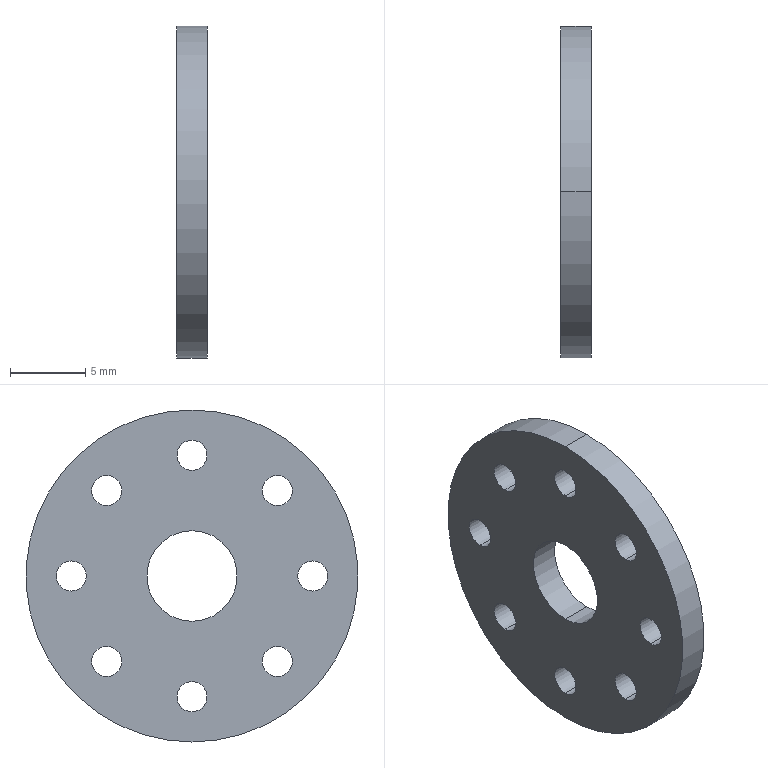Part | SolidWorks | features BaseBody 1 | 1 solid | 22 faces | box 2 x 22 x 22 mm | volume 653.451 mm3 | cylinder 20 | plane 2 | commonest cylinder face diameters 2 x16 6 x2 22 x2
STEP:
#1=CARTESIAN_POINT('',(1.,5.657,4.657));
#2=VERTEX_POINT('',#1);
#3=CARTESIAN_POINT('',(1.,5.657,6.657));
#4=VERTEX_POINT('',#3);
#5=CARTESIAN_POINT('',(1.,5.657,5.657));
#6=DIRECTION('',(-1.,0.,0.));
#7=DIRECTION('',(0.,-0.7071,0.7071));
#8=AXIS2_PLACEMENT_3D('',#5,#6,#7);
#9=CIRCLE('',#8,1.);
#10=EDGE_CURVE('',#2,#4,#9,.T.);
#11=ORIENTED_EDGE('',*,*,#10,.F.);
#12=CARTESIAN_POINT('',(-1.,5.657,4.657));
#13=VERTEX_POINT('',#12);
#14=CARTESIAN_POINT('',(1.,5.657,4.657));
#15=DIRECTION('',(-1.,0.,0.));
#16=VECTOR('',#15,1000.);
#17=LINE('',#14,#16);
#18=EDGE_CURVE('',#2,#13,#17,.T.);
#19=ORIENTED_EDGE('',*,*,#18,.T.);
#20=CARTESIAN_POINT('',(-1.,5.657,6.657));
#21=VERTEX_POINT('',#20);
#22=CARTESIAN_POINT('',(-1.,5.657,5.657));
#23=DIRECTION('',(-1.,0.,0.));
#24=DIRECTION('',(0.,-0.7071,0.7071));
#25=AXIS2_PLACEMENT_3D('',#22,#23,#24);
#26=CIRCLE('',#25,1.);
#27=EDGE_CURVE('',#13,#21,#26,.T.);
#28=ORIENTED_EDGE('',*,*,#27,.T.);
#29=CARTESIAN_POINT('',(1.,5.657,6.657));
#30=DIRECTION('',(-1.,0.,0.));
#31=VECTOR('',#30,1000.);
#32=LINE('',#29,#31);
#33=EDGE_CURVE('',#4,#21,#32,.T.);
#34=ORIENTED_EDGE('',*,*,#33,.F.);
#35=EDGE_LOOP('',(#11,#19,#28,#34));
#36=FACE_OUTER_BOUND('',#35,.T.);
#37=CARTESIAN_POINT('',(1.,5.657,5.657));
#38=DIRECTION('',(-1.,0.,0.));
#39=DIRECTION('',(0.,0.,1.));
#40=AXIS2_PLACEMENT_3D('',#37,#38,#39);
#41=CYLINDRICAL_SURFACE('',#40,1.);
#42=ADVANCED_FACE('',(#36),#41,.F.);
#43=CARTESIAN_POINT('',(1.,0.,7.));
#44=VERTEX_POINT('',#43);
#45=CARTESIAN_POINT('',(1.,0.,9.));
#46=VERTEX_POINT('',#45);
#47=CARTESIAN_POINT('',(1.,0.,8.));
#48=DIRECTION('',(-1.,0.,0.));
#49=DIRECTION('',(0.,-1.,0.));
#50=AXIS2_PLACEMENT_3D('',#47,#48,#49);
#51=CIRCLE('',#50,1.);
#52=EDGE_CURVE('',#44,#46,#51,.T.);
#53=ORIENTED_EDGE('',*,*,#52,.F.);
#54=CARTESIAN_POINT('',(-1.,0.,7.));
#55=VERTEX_POINT('',#54);
#56=CARTESIAN_POINT('',(1.,0.,7.));
#57=DIRECTION('',(-1.,0.,0.));
#58=VECTOR('',#57,1000.);
#59=LINE('',#56,#58);
#60=EDGE_CURVE('',#44,#55,#59,.T.);
#61=ORIENTED_EDGE('',*,*,#60,.T.);
#62=CARTESIAN_POINT('',(-1.,0.,9.));
#63=VERTEX_POINT('',#62);
#64=CARTESIAN_POINT('',(-1.,0.,8.));
#65=DIRECTION('',(-1.,0.,0.));
#66=DIRECTION('',(0.,-1.,0.));
#67=AXIS2_PLACEMENT_3D('',#64,#65,#66);
#68=CIRCLE('',#67,1.);
#69=EDGE_CURVE('',#55,#63,#68,.T.);
#70=ORIENTED_EDGE('',*,*,#69,.T.);
#71=CARTESIAN_POINT('',(1.,0.,9.));
#72=DIRECTION('',(-1.,0.,0.));
#73=VECTOR('',#72,1000.);
#74=LINE('',#71,#73);
#75=EDGE_CURVE('',#46,#63,#74,.T.);
#76=ORIENTED_EDGE('',*,*,#75,.F.);
#77=EDGE_LOOP('',(#53,#61,#70,#76));
#78=FACE_OUTER_BOUND('',#77,.T.);
#79=CARTESIAN_POINT('',(1.,0.,8.));
#80=DIRECTION('',(-1.,0.,0.));
#81=DIRECTION('',(0.,0.,1.));
#82=AXIS2_PLACEMENT_3D('',#79,#80,#81);
#83=CYLINDRICAL_SURFACE('',#82,1.);
#84=ADVANCED_FACE('',(#78),#83,.F.);
#85=CARTESIAN_POINT('',(1.,-5.657,4.657));
#86=VERTEX_POINT('',#85);
#87=CARTESIAN_POINT('',(1.,-5.657,6.657));
#88=VERTEX_POINT('',#87);
#89=CARTESIAN_POINT('',(1.,-5.657,5.657));
#90=DIRECTION('',(-1.,0.,0.));
#91=DIRECTION('',(0.,-0.7071,-0.7071));
#92=AXIS2_PLACEMENT_3D('',#89,#90,#91);
#93=CIRCLE('',#92,1.);
#94=EDGE_CURVE('',#86,#88,#93,.T.);
#95=ORIENTED_EDGE('',*,*,#94,.F.);
#96=CARTESIAN_POINT('',(-1.,-5.657,4.657));
#97=VERTEX_POINT('',#96);
#98=CARTESIAN_POINT('',(1.,-5.657,4.657));
#99=DIRECTION('',(-1.,0.,0.));
#100=VECTOR('',#99,1000.);
#101=LINE('',#98,#100);
#102=EDGE_CURVE('',#86,#97,#101,.T.);
#103=ORIENTED_EDGE('',*,*,#102,.T.);
#104=CARTESIAN_POINT('',(-1.,-5.657,6.657));
#105=VERTEX_POINT('',#104);
#106=CARTESIAN_POINT('',(-1.,-5.657,5.657));
#107=DIRECTION('',(-1.,0.,0.));
#108=DIRECTION('',(0.,-0.7071,-0.7071));
#109=AXIS2_PLACEMENT_3D('',#106,#107,#108);
#110=CIRCLE('',#109,1.);
#111=EDGE_CURVE('',#97,#105,#110,.T.);
#112=ORIENTED_EDGE('',*,*,#111,.T.);
#113=CARTESIAN_POINT('',(1.,-5.657,6.657));
#114=DIRECTION('',(-1.,0.,0.));
#115=VECTOR('',#114,1000.);
#116=LINE('',#113,#115);
#117=EDGE_CURVE('',#88,#105,#116,.T.);
#118=ORIENTED_EDGE('',*,*,#117,.F.);
#119=EDGE_LOOP('',(#95,#103,#112,#118));
#120=FACE_OUTER_BOUND('',#119,.T.);
#121=CARTESIAN_POINT('',(1.,-5.657,5.657));
#122=DIRECTION('',(-1.,0.,0.));
#123=DIRECTION('',(0.,0.,1.));
#124=AXIS2_PLACEMENT_3D('',#121,#122,#123);
#125=CYLINDRICAL_SURFACE('',#124,1.);
#126=ADVANCED_FACE('',(#120),#125,.F.);
#127=CARTESIAN_POINT('',(1.,-8.,-1.));
#128=VERTEX_POINT('',#127);
#129=CARTESIAN_POINT('',(1.,-8.,1.));
#130=VERTEX_POINT('',#129);
#131=CARTESIAN_POINT('',(1.,-8.,0.));
#132=DIRECTION('',(-1.,0.,0.));
#133=DIRECTION('',(0.,0.,-1.));
#134=AXIS2_PLACEMENT_3D('',#131,#132,#133);
#135=CIRCLE('',#134,1.);
#136=EDGE_CURVE('',#128,#130,#135,.T.);
#137=ORIENTED_EDGE('',*,*,#136,.F.);
#138=CARTESIAN_POINT('',(-1.,-8.,-1.));
#139=VERTEX_POINT('',#138);
#140=CARTESIAN_POINT('',(1.,-8.,-1.));
#141=DIRECTION('',(-1.,0.,0.));
#142=VECTOR('',#141,1000.);
#143=LINE('',#140,#142);
#144=EDGE_CURVE('',#128,#139,#143,.T.);
#145=ORIENTED_EDGE('',*,*,#144,.T.);
#146=CARTESIAN_POINT('',(-1.,-8.,1.));
#147=VERTEX_POINT('',#146);
#148=CARTESIAN_POINT('',(-1.,-8.,0.));
#149=DIRECTION('',(-1.,0.,0.));
#150=DIRECTION('',(0.,0.,-1.));
#151=AXIS2_PLACEMENT_3D('',#148,#149,#150);
#152=CIRCLE('',#151,1.);
#153=EDGE_CURVE('',#139,#147,#152,.T.);
#154=ORIENTED_EDGE('',*,*,#153,.T.);
#155=CARTESIAN_POINT('',(1.,-8.,1.));
#156=DIRECTION('',(-1.,0.,0.));
#157=VECTOR('',#156,1000.);
#158=LINE('',#155,#157);
#159=EDGE_CURVE('',#130,#147,#158,.T.);
#160=ORIENTED_EDGE('',*,*,#159,.F.);
#161=EDGE_LOOP('',(#137,#145,#154,#160));
#162=FACE_OUTER_BOUND('',#161,.T.);
#163=CARTESIAN_POINT('',(1.,-8.,0.));
#164=DIRECTION('',(-1.,0.,0.));
#165=DIRECTION('',(0.,0.,1.));
#166=AXIS2_PLACEMENT_3D('',#163,#164,#165);
#167=CYLINDRICAL_SURFACE('',#166,1.);
#168=ADVANCED_FACE('',(#162),#167,.F.);
#169=CARTESIAN_POINT('',(1.,-5.657,-6.657));
#170=VERTEX_POINT('',#169);
#171=CARTESIAN_POINT('',(1.,-5.657,-4.657));
#172=VERTEX_POINT('',#171);
#173=CARTESIAN_POINT('',(1.,-5.657,-5.657));
#174=DIRECTION('',(-1.,0.,0.));
#175=DIRECTION('',(0.,0.7071,-0.7071));
#176=AXIS2_PLACEMENT_3D('',#173,#174,#175);
#177=CIRCLE('',#176,1.);
#178=EDGE_CURVE('',#170,#172,#177,.T.);
#179=ORIENTED_EDGE('',*,*,#178,.F.);
#180=CARTESIAN_POINT('',(-1.,-5.657,-6.657));
#181=VERTEX_POINT('',#180);
#182=CARTESIAN_POINT('',(1.,-5.657,-6.657));
#183=DIRECTION('',(-1.,0.,0.));
#184=VECTOR('',#183,1000.);
#185=LINE('',#182,#184);
#186=EDGE_CURVE('',#170,#181,#185,.T.);
#187=ORIENTED_EDGE('',*,*,#186,.T.);
#188=CARTESIAN_POINT('',(-1.,-5.657,-4.657));
#189=VERTEX_POINT('',#188);
#190=CARTESIAN_POINT('',(-1.,-5.657,-5.657));
#191=DIRECTION('',(-1.,0.,0.));
#192=DIRECTION('',(0.,0.7071,-0.7071));
#193=AXIS2_PLACEMENT_3D('',#190,#191,#192);
#194=CIRCLE('',#193,1.);
#195=EDGE_CURVE('',#181,#189,#194,.T.);
#196=ORIENTED_EDGE('',*,*,#195,.T.);
#197=CARTESIAN_POINT('',(1.,-5.657,-4.657));
#198=DIRECTION('',(-1.,0.,0.));
#199=VECTOR('',#198,1000.);
#200=LINE('',#197,#199);
#201=EDGE_CURVE('',#172,#189,#200,.T.);
#202=ORIENTED_EDGE('',*,*,#201,.F.);
#203=EDGE_LOOP('',(#179,#187,#196,#202));
#204=FACE_OUTER_BOUND('',#203,.T.);
#205=CARTESIAN_POINT('',(1.,-5.657,-5.657));
#206=DIRECTION('',(-1.,0.,0.));
#207=DIRECTION('',(0.,0.,1.));
#208=AXIS2_PLACEMENT_3D('',#205,#206,#207);
#209=CYLINDRICAL_SURFACE('',#208,1.);
#210=ADVANCED_FACE('',(#204),#209,.F.);
#211=CARTESIAN_POINT('',(1.,0.,-9.));
#212=VERTEX_POINT('',#211);
#213=CARTESIAN_POINT('',(1.,0.,-7.));
#214=VERTEX_POINT('',#213);
#215=CARTESIAN_POINT('',(1.,0.,-8.));
#216=DIRECTION('',(-1.,0.,0.));
#217=DIRECTION('',(0.,1.,0.));
#218=AXIS2_PLACEMENT_3D('',#215,#216,#217);
#219=CIRCLE('',#218,1.);
#220=EDGE_CURVE('',#212,#214,#219,.T.);
#221=ORIENTED_EDGE('',*,*,#220,.F.);
#222=CARTESIAN_POINT('',(-1.,0.,-9.));
#223=VERTEX_POINT('',#222);
#224=CARTESIAN_POINT('',(1.,0.,-9.));
#225=DIRECTION('',(-1.,0.,0.));
#226=VECTOR('',#225,1000.);
#227=LINE('',#224,#226);
#228=EDGE_CURVE('',#212,#223,#227,.T.);
#229=ORIENTED_EDGE('',*,*,#228,.T.);
#230=CARTESIAN_POINT('',(-1.,0.,-7.));
#231=VERTEX_POINT('',#230);
#232=CARTESIAN_POINT('',(-1.,0.,-8.));
#233=DIRECTION('',(-1.,0.,0.));
#234=DIRECTION('',(0.,1.,0.));
#235=AXIS2_PLACEMENT_3D('',#232,#233,#234);
#236=CIRCLE('',#235,1.);
#237=EDGE_CURVE('',#223,#231,#236,.T.);
#238=ORIENTED_EDGE('',*,*,#237,.T.);
#239=CARTESIAN_POINT('',(1.,0.,-7.));
#240=DIRECTION('',(-1.,0.,0.));
#241=VECTOR('',#240,1000.);
#242=LINE('',#239,#241);
#243=EDGE_CURVE('',#214,#231,#242,.T.);
#244=ORIENTED_EDGE('',*,*,#243,.F.);
#245=EDGE_LOOP('',(#221,#229,#238,#244));
#246=FACE_OUTER_BOUND('',#245,.T.);
#247=CARTESIAN_POINT('',(1.,0.,-8.));
#248=DIRECTION('',(-1.,0.,0.));
#249=DIRECTION('',(0.,0.,1.));
#250=AXIS2_PLACEMENT_3D('',#247,#248,#249);
#251=CYLINDRICAL_SURFACE('',#250,1.);
#252=ADVANCED_FACE('',(#246),#251,.F.);
#253=CARTESIAN_POINT('',(1.,5.657,-6.657));
#254=VERTEX_POINT('',#253);
#255=CARTESIAN_POINT('',(1.,5.657,-4.657));
#256=VERTEX_POINT('',#255);
#257=CARTESIAN_POINT('',(1.,5.657,-5.657));
#258=DIRECTION('',(-1.,0.,0.));
#259=DIRECTION('',(0.,0.7071,0.7071));
#260=AXIS2_PLACEMENT_3D('',#257,#258,#259);
#261=CIRCLE('',#260,1.);
#262=EDGE_CURVE('',#254,#256,#261,.T.);
#263=ORIENTED_EDGE('',*,*,#262,.F.);
#264=CARTESIAN_POINT('',(-1.,5.657,-6.657));
#265=VERTEX_POINT('',#264);
#266=CARTESIAN_POINT('',(1.,5.657,-6.657));
#267=DIRECTION('',(-1.,0.,0.));
#268=VECTOR('',#267,1000.);
#269=LINE('',#266,#268);
#270=EDGE_CURVE('',#254,#265,#269,.T.);
#271=ORIENTED_EDGE('',*,*,#270,.T.);
#272=CARTESIAN_POINT('',(-1.,5.657,-4.657));
#273=VERTEX_POINT('',#272);
#274=CARTESIAN_POINT('',(-1.,5.657,-5.657));
#275=DIRECTION('',(-1.,0.,0.));
#276=DIRECTION('',(0.,0.7071,0.7071));
#277=AXIS2_PLACEMENT_3D('',#274,#275,#276);
#278=CIRCLE('',#277,1.);
#279=EDGE_CURVE('',#265,#273,#278,.T.);
#280=ORIENTED_EDGE('',*,*,#279,.T.);
#281=CARTESIAN_POINT('',(1.,5.657,-4.657));
#282=DIRECTION('',(-1.,0.,0.));
#283=VECTOR('',#282,1000.);
#284=LINE('',#281,#283);
#285=EDGE_CURVE('',#256,#273,#284,.T.);
#286=ORIENTED_EDGE('',*,*,#285,.F.);
#287=EDGE_LOOP('',(#263,#271,#280,#286));
#288=FACE_OUTER_BOUND('',#287,.T.);
#289=CARTESIAN_POINT('',(1.,5.657,-5.657));
#290=DIRECTION('',(-1.,0.,0.));
#291=DIRECTION('',(0.,0.,1.));
#292=AXIS2_PLACEMENT_3D('',#289,#290,#291);
#293=CYLINDRICAL_SURFACE('',#292,1.);
#294=ADVANCED_FACE('',(#288),#293,.F.);
#295=CARTESIAN_POINT('',(1.,8.,-1.));
#296=VERTEX_POINT('',#295);
#297=CARTESIAN_POINT('',(1.,8.,1.));
#298=VERTEX_POINT('',#297);
#299=CARTESIAN_POINT('',(1.,8.,0.));
#300=DIRECTION('',(-1.,0.,0.));
#301=DIRECTION('',(0.,0.,1.));
#302=AXIS2_PLACEMENT_3D('',#299,#300,#301);
#303=CIRCLE('',#302,1.);
#304=EDGE_CURVE('',#296,#298,#303,.T.);
#305=ORIENTED_EDGE('',*,*,#304,.F.);
#306=CARTESIAN_POINT('',(-1.,8.,-1.));
#307=VERTEX_POINT('',#306);
#308=CARTESIAN_POINT('',(1.,8.,-1.));
#309=DIRECTION('',(-1.,0.,0.));
#310=VECTOR('',#309,1000.);
#311=LINE('',#308,#310);
#312=EDGE_CURVE('',#296,#307,#311,.T.);
#313=ORIENTED_EDGE('',*,*,#312,.T.);
#314=CARTESIAN_POINT('',(-1.,8.,1.));
#315=VERTEX_POINT('',#314);
#316=CARTESIAN_POINT('',(-1.,8.,0.));
#317=DIRECTION('',(-1.,0.,0.));
#318=DIRECTION('',(0.,0.,1.));
#319=AXIS2_PLACEMENT_3D('',#316,#317,#318);
#320=CIRCLE('',#319,1.);
#321=EDGE_CURVE('',#307,#315,#320,.T.);
#322=ORIENTED_EDGE('',*,*,#321,.T.);
#323=CARTESIAN_POINT('',(1.,8.,1.));
#324=DIRECTION('',(-1.,0.,0.));
#325=VECTOR('',#324,1000.);
#326=LINE('',#323,#325);
#327=EDGE_CURVE('',#298,#315,#326,.T.);
#328=ORIENTED_EDGE('',*,*,#327,.F.);
#329=EDGE_LOOP('',(#305,#313,#322,#328));
#330=FACE_OUTER_BOUND('',#329,.T.);
#331=CARTESIAN_POINT('',(1.,8.,0.));
#332=DIRECTION('',(-1.,0.,0.));
#333=DIRECTION('',(0.,0.,1.));
#334=AXIS2_PLACEMENT_3D('',#331,#332,#333);
#335=CYLINDRICAL_SURFACE('',#334,1.);
#336=ADVANCED_FACE('',(#330),#335,.F.);
#337=CARTESIAN_POINT('',(1.,0.,11.));
#338=VERTEX_POINT('',#337);
#339=CARTESIAN_POINT('',(1.,0.,-11.));
#340=VERTEX_POINT('',#339);
#341=CARTESIAN_POINT('',(1.,0.,0.));
#342=DIRECTION('',(-1.,0.,0.));
#343=DIRECTION('',(0.,0.,1.));
#344=AXIS2_PLACEMENT_3D('',#341,#342,#343);
#345=CIRCLE('',#344,11.);
#346=EDGE_CURVE('',#338,#340,#345,.T.);
#347=ORIENTED_EDGE('',*,*,#346,.T.);
#348=CARTESIAN_POINT('',(-1.,0.,-11.));
#349=VERTEX_POINT('',#348);
#350=CARTESIAN_POINT('',(0.,0.,-11.));
#351=DIRECTION('',(-1.,0.,0.));
#352=VECTOR('',#351,1000.);
#353=LINE('',#350,#352);
#354=EDGE_CURVE('',#340,#349,#353,.T.);
#355=ORIENTED_EDGE('',*,*,#354,.T.);
#356=CARTESIAN_POINT('',(-1.,0.,11.));
#357=VERTEX_POINT('',#356);
#358=CARTESIAN_POINT('',(-1.,0.,0.));
#359=DIRECTION('',(-1.,0.,0.));
#360=DIRECTION('',(0.,0.,1.));
#361=AXIS2_PLACEMENT_3D('',#358,#359,#360);
#362=CIRCLE('',#361,11.);
#363=EDGE_CURVE('',#357,#349,#362,.T.);
#364=ORIENTED_EDGE('',*,*,#363,.F.);
#365=CARTESIAN_POINT('',(0.,0.,11.));
#366=DIRECTION('',(-1.,0.,0.));
#367=VECTOR('',#366,1000.);
#368=LINE('',#365,#367);
#369=EDGE_CURVE('',#338,#357,#368,.T.);
#370=ORIENTED_EDGE('',*,*,#369,.F.);
#371=EDGE_LOOP('',(#347,#355,#364,#370));
#372=FACE_OUTER_BOUND('',#371,.T.);
#373=CARTESIAN_POINT('',(0.,0.,0.));
#374=DIRECTION('',(-1.,0.,0.));
#375=DIRECTION('',(0.,0.,1.));
#376=AXIS2_PLACEMENT_3D('',#373,#374,#375);
#377=CYLINDRICAL_SURFACE('',#376,11.);
#378=ADVANCED_FACE('',(#372),#377,.T.);
#379=CARTESIAN_POINT('',(1.,0.,-3.));
#380=VERTEX_POINT('',#379);
#381=CARTESIAN_POINT('',(1.,0.,3.));
#382=VERTEX_POINT('',#381);
#383=CARTESIAN_POINT('',(1.,0.,0.));
#384=DIRECTION('',(-1.,0.,0.));
#385=DIRECTION('',(0.,0.,1.));
#386=AXIS2_PLACEMENT_3D('',#383,#384,#385);
#387=CIRCLE('',#386,3.);
#388=EDGE_CURVE('',#380,#382,#387,.T.);
#389=ORIENTED_EDGE('',*,*,#388,.F.);
#390=CARTESIAN_POINT('',(-1.,0.,-3.));
#391=VERTEX_POINT('',#390);
#392=CARTESIAN_POINT('',(0.,0.,-3.));
#393=DIRECTION('',(-1.,0.,0.));
#394=VECTOR('',#393,1000.);
#395=LINE('',#392,#394);
#396=EDGE_CURVE('',#380,#391,#395,.T.);
#397=ORIENTED_EDGE('',*,*,#396,.T.);
#398=CARTESIAN_POINT('',(-1.,0.,3.));
#399=VERTEX_POINT('',#398);
#400=CARTESIAN_POINT('',(-1.,0.,0.));
#401=DIRECTION('',(-1.,0.,0.));
#402=DIRECTION('',(0.,0.,1.));
#403=AXIS2_PLACEMENT_3D('',#400,#401,#402);
#404=CIRCLE('',#403,3.);
#405=EDGE_CURVE('',#391,#399,#404,.T.);
#406=ORIENTED_EDGE('',*,*,#405,.T.);
#407=CARTESIAN_POINT('',(0.,0.,3.));
#408=DIRECTION('',(-1.,0.,0.));
#409=VECTOR('',#408,1000.);
#410=LINE('',#407,#409);
#411=EDGE_CURVE('',#382,#399,#410,.T.);
#412=ORIENTED_EDGE('',*,*,#411,.F.);
#413=EDGE_LOOP('',(#389,#397,#406,#412));
#414=FACE_OUTER_BOUND('',#413,.T.);
#415=CARTESIAN_POINT('',(0.,0.,0.));
#416=DIRECTION('',(-1.,0.,0.));
#417=DIRECTION('',(0.,0.,1.));
#418=AXIS2_PLACEMENT_3D('',#415,#416,#417);
#419=CYLINDRICAL_SURFACE('',#418,3.);
#420=ADVANCED_FACE('',(#414),#419,.F.);
#421=ORIENTED_EDGE('',*,*,#396,.F.);
#422=CARTESIAN_POINT('',(1.,0.,0.));
#423=DIRECTION('',(-1.,0.,0.));
#424=DIRECTION('',(0.,0.,1.));
#425=AXIS2_PLACEMENT_3D('',#422,#423,#424);
#426=CIRCLE('',#425,3.);
#427=EDGE_CURVE('',#382,#380,#426,.T.);
#428=ORIENTED_EDGE('',*,*,#427,.F.);
#429=ORIENTED_EDGE('',*,*,#411,.T.);
#430=CARTESIAN_POINT('',(-1.,0.,0.));
#431=DIRECTION('',(-1.,0.,0.));
#432=DIRECTION('',(0.,0.,1.));
#433=AXIS2_PLACEMENT_3D('',#430,#431,#432);
#434=CIRCLE('',#433,3.);
#435=EDGE_CURVE('',#399,#391,#434,.T.);
#436=ORIENTED_EDGE('',*,*,#435,.T.);
#437=EDGE_LOOP('',(#421,#428,#429,#436));
#438=FACE_OUTER_BOUND('',#437,.T.);
#439=CARTESIAN_POINT('',(0.,0.,0.));
#440=DIRECTION('',(-1.,0.,0.));
#441=DIRECTION('',(0.,0.,1.));
#442=AXIS2_PLACEMENT_3D('',#439,#440,#441);
#443=CYLINDRICAL_SURFACE('',#442,3.);
#444=ADVANCED_FACE('',(#438),#443,.F.);
#445=CARTESIAN_POINT('',(-1.,5.657,5.657));
#446=DIRECTION('',(-1.,0.,0.));
#447=DIRECTION('',(0.,-0.7071,0.7071));
#448=AXIS2_PLACEMENT_3D('',#445,#446,#447);
#449=CIRCLE('',#448,1.);
#450=EDGE_CURVE('',#21,#13,#449,.T.);
#451=ORIENTED_EDGE('',*,*,#450,.F.);
#452=ORIENTED_EDGE('',*,*,#27,.F.);
#453=EDGE_LOOP('',(#451,#452));
#454=FACE_BOUND('',#453,.T.);
#455=CARTESIAN_POINT('',(-1.,0.,8.));
#456=DIRECTION('',(-1.,0.,0.));
#457=DIRECTION('',(0.,-1.,0.));
#458=AXIS2_PLACEMENT_3D('',#455,#456,#457);
#459=CIRCLE('',#458,1.);
#460=EDGE_CURVE('',#63,#55,#459,.T.);
#461=ORIENTED_EDGE('',*,*,#460,.F.);
#462=ORIENTED_EDGE('',*,*,#69,.F.);
#463=EDGE_LOOP('',(#461,#462));
#464=FACE_BOUND('',#463,.T.);
#465=CARTESIAN_POINT('',(-1.,-5.657,5.657));
#466=DIRECTION('',(-1.,0.,0.));
#467=DIRECTION('',(0.,-0.7071,-0.7071));
#468=AXIS2_PLACEMENT_3D('',#465,#466,#467);
#469=CIRCLE('',#468,1.);
#470=EDGE_CURVE('',#105,#97,#469,.T.);
#471=ORIENTED_EDGE('',*,*,#470,.F.);
#472=ORIENTED_EDGE('',*,*,#111,.F.);
#473=EDGE_LOOP('',(#471,#472));
#474=FACE_BOUND('',#473,.T.);
#475=CARTESIAN_POINT('',(-1.,-8.,0.));
#476=DIRECTION('',(-1.,0.,0.));
#477=DIRECTION('',(0.,0.,-1.));
#478=AXIS2_PLACEMENT_3D('',#475,#476,#477);
#479=CIRCLE('',#478,1.);
#480=EDGE_CURVE('',#147,#139,#479,.T.);
#481=ORIENTED_EDGE('',*,*,#480,.F.);
#482=ORIENTED_EDGE('',*,*,#153,.F.);
#483=EDGE_LOOP('',(#481,#482));
#484=FACE_BOUND('',#483,.T.);
#485=CARTESIAN_POINT('',(-1.,-5.657,-5.657));
#486=DIRECTION('',(-1.,0.,0.));
#487=DIRECTION('',(0.,0.7071,-0.7071));
#488=AXIS2_PLACEMENT_3D('',#485,#486,#487);
#489=CIRCLE('',#488,1.);
#490=EDGE_CURVE('',#189,#181,#489,.T.);
#491=ORIENTED_EDGE('',*,*,#490,.F.);
#492=ORIENTED_EDGE('',*,*,#195,.F.);
#493=EDGE_LOOP('',(#491,#492));
#494=FACE_BOUND('',#493,.T.);
#495=CARTESIAN_POINT('',(-1.,0.,-8.));
#496=DIRECTION('',(-1.,0.,0.));
#497=DIRECTION('',(0.,1.,0.));
#498=AXIS2_PLACEMENT_3D('',#495,#496,#497);
#499=CIRCLE('',#498,1.);
#500=EDGE_CURVE('',#231,#223,#499,.T.);
#501=ORIENTED_EDGE('',*,*,#500,.F.);
#502=ORIENTED_EDGE('',*,*,#237,.F.);
#503=EDGE_LOOP('',(#501,#502));
#504=FACE_BOUND('',#503,.T.);
#505=CARTESIAN_POINT('',(-1.,5.657,-5.657));
#506=DIRECTION('',(-1.,0.,0.));
#507=DIRECTION('',(0.,0.7071,0.7071));
#508=AXIS2_PLACEMENT_3D('',#505,#506,#507);
#509=CIRCLE('',#508,1.);
#510=EDGE_CURVE('',#273,#265,#509,.T.);
#511=ORIENTED_EDGE('',*,*,#510,.F.);
#512=ORIENTED_EDGE('',*,*,#279,.F.);
#513=EDGE_LOOP('',(#511,#512));
#514=FACE_BOUND('',#513,.T.);
#515=CARTESIAN_POINT('',(-1.,8.,0.));
#516=DIRECTION('',(-1.,0.,0.));
#517=DIRECTION('',(0.,0.,1.));
#518=AXIS2_PLACEMENT_3D('',#515,#516,#517);
#519=CIRCLE('',#518,1.);
#520=EDGE_CURVE('',#315,#307,#519,.T.);
#521=ORIENTED_EDGE('',*,*,#520,.F.);
#522=ORIENTED_EDGE('',*,*,#321,.F.);
#523=EDGE_LOOP('',(#521,#522));
#524=FACE_BOUND('',#523,.T.);
#525=ORIENTED_EDGE('',*,*,#435,.F.);
#526=ORIENTED_EDGE('',*,*,#405,.F.);
#527=EDGE_LOOP('',(#525,#526));
#528=FACE_BOUND('',#527,.T.);
#529=ORIENTED_EDGE('',*,*,#363,.T.);
#530=CARTESIAN_POINT('',(-1.,0.,0.));
#531=DIRECTION('',(-1.,0.,0.));
#532=DIRECTION('',(0.,0.,1.));
#533=AXIS2_PLACEMENT_3D('',#530,#531,#532);
#534=CIRCLE('',#533,11.);
#535=EDGE_CURVE('',#349,#357,#534,.T.);
#536=ORIENTED_EDGE('',*,*,#535,.T.);
#537=EDGE_LOOP('',(#529,#536));
#538=FACE_OUTER_BOUND('',#537,.T.);
#539=CARTESIAN_POINT('',(-1.,3.,0.));
#540=DIRECTION('',(1.,0.,0.));
#541=DIRECTION('',(0.,0.,-1.));
#542=AXIS2_PLACEMENT_3D('',#539,#540,#541);
#543=PLANE('',#542);
#544=ADVANCED_FACE('',(#454,#464,#474,#484,#494,#504,#514,#524,#528,#538),#543,.F.);
#545=ORIENTED_EDGE('',*,*,#354,.F.);
#546=CARTESIAN_POINT('',(1.,0.,0.));
#547=DIRECTION('',(-1.,0.,0.));
#548=DIRECTION('',(0.,0.,1.));
#549=AXIS2_PLACEMENT_3D('',#546,#547,#548);
#550=CIRCLE('',#549,11.);
#551=EDGE_CURVE('',#340,#338,#550,.T.);
#552=ORIENTED_EDGE('',*,*,#551,.T.);
#553=ORIENTED_EDGE('',*,*,#369,.T.);
#554=ORIENTED_EDGE('',*,*,#535,.F.);
#555=EDGE_LOOP('',(#545,#552,#553,#554));
#556=FACE_OUTER_BOUND('',#555,.T.);
#557=CARTESIAN_POINT('',(0.,0.,0.));
#558=DIRECTION('',(-1.,0.,0.));
#559=DIRECTION('',(0.,0.,1.));
#560=AXIS2_PLACEMENT_3D('',#557,#558,#559);
#561=CYLINDRICAL_SURFACE('',#560,11.);
#562=ADVANCED_FACE('',(#556),#561,.T.);
#563=CARTESIAN_POINT('',(1.,5.657,5.657));
#564=DIRECTION('',(-1.,0.,0.));
#565=DIRECTION('',(0.,-0.7071,0.7071));
#566=AXIS2_PLACEMENT_3D('',#563,#564,#565);
#567=CIRCLE('',#566,1.);
#568=EDGE_CURVE('',#4,#2,#567,.T.);
#569=ORIENTED_EDGE('',*,*,#568,.T.);
#570=ORIENTED_EDGE('',*,*,#10,.T.);
#571=EDGE_LOOP('',(#569,#570));
#572=FACE_BOUND('',#571,.T.);
#573=CARTESIAN_POINT('',(1.,0.,8.));
#574=DIRECTION('',(-1.,0.,0.));
#575=DIRECTION('',(0.,-1.,0.));
#576=AXIS2_PLACEMENT_3D('',#573,#574,#575);
#577=CIRCLE('',#576,1.);
#578=EDGE_CURVE('',#46,#44,#577,.T.);
#579=ORIENTED_EDGE('',*,*,#578,.T.);
#580=ORIENTED_EDGE('',*,*,#52,.T.);
#581=EDGE_LOOP('',(#579,#580));
#582=FACE_BOUND('',#581,.T.);
#583=CARTESIAN_POINT('',(1.,-5.657,5.657));
#584=DIRECTION('',(-1.,0.,0.));
#585=DIRECTION('',(0.,-0.7071,-0.7071));
#586=AXIS2_PLACEMENT_3D('',#583,#584,#585);
#587=CIRCLE('',#586,1.);
#588=EDGE_CURVE('',#88,#86,#587,.T.);
#589=ORIENTED_EDGE('',*,*,#588,.T.);
#590=ORIENTED_EDGE('',*,*,#94,.T.);
#591=EDGE_LOOP('',(#589,#590));
#592=FACE_BOUND('',#591,.T.);
#593=CARTESIAN_POINT('',(1.,-8.,0.));
#594=DIRECTION('',(-1.,0.,0.));
#595=DIRECTION('',(0.,0.,-1.));
#596=AXIS2_PLACEMENT_3D('',#593,#594,#595);
#597=CIRCLE('',#596,1.);
#598=EDGE_CURVE('',#130,#128,#597,.T.);
#599=ORIENTED_EDGE('',*,*,#598,.T.);
#600=ORIENTED_EDGE('',*,*,#136,.T.);
#601=EDGE_LOOP('',(#599,#600));
#602=FACE_BOUND('',#601,.T.);
#603=CARTESIAN_POINT('',(1.,-5.657,-5.657));
#604=DIRECTION('',(-1.,0.,0.));
#605=DIRECTION('',(0.,0.7071,-0.7071));
#606=AXIS2_PLACEMENT_3D('',#603,#604,#605);
#607=CIRCLE('',#606,1.);
#608=EDGE_CURVE('',#172,#170,#607,.T.);
#609=ORIENTED_EDGE('',*,*,#608,.T.);
#610=ORIENTED_EDGE('',*,*,#178,.T.);
#611=EDGE_LOOP('',(#609,#610));
#612=FACE_BOUND('',#611,.T.);
#613=CARTESIAN_POINT('',(1.,0.,-8.));
#614=DIRECTION('',(-1.,0.,0.));
#615=DIRECTION('',(0.,1.,0.));
#616=AXIS2_PLACEMENT_3D('',#613,#614,#615);
#617=CIRCLE('',#616,1.);
#618=EDGE_CURVE('',#214,#212,#617,.T.);
#619=ORIENTED_EDGE('',*,*,#618,.T.);
#620=ORIENTED_EDGE('',*,*,#220,.T.);
#621=EDGE_LOOP('',(#619,#620));
#622=FACE_BOUND('',#621,.T.);
#623=CARTESIAN_POINT('',(1.,5.657,-5.657));
#624=DIRECTION('',(-1.,0.,0.));
#625=DIRECTION('',(0.,0.7071,0.7071));
#626=AXIS2_PLACEMENT_3D('',#623,#624,#625);
#627=CIRCLE('',#626,1.);
#628=EDGE_CURVE('',#256,#254,#627,.T.);
#629=ORIENTED_EDGE('',*,*,#628,.T.);
#630=ORIENTED_EDGE('',*,*,#262,.T.);
#631=EDGE_LOOP('',(#629,#630));
#632=FACE_BOUND('',#631,.T.);
#633=CARTESIAN_POINT('',(1.,8.,0.));
#634=DIRECTION('',(-1.,0.,0.));
#635=DIRECTION('',(0.,0.,1.));
#636=AXIS2_PLACEMENT_3D('',#633,#634,#635);
#637=CIRCLE('',#636,1.);
#638=EDGE_CURVE('',#298,#296,#637,.T.);
#639=ORIENTED_EDGE('',*,*,#638,.T.);
#640=ORIENTED_EDGE('',*,*,#304,.T.);
#641=EDGE_LOOP('',(#639,#640));
#642=FACE_BOUND('',#641,.T.);
#643=ORIENTED_EDGE('',*,*,#346,.F.);
#644=ORIENTED_EDGE('',*,*,#551,.F.);
#645=EDGE_LOOP('',(#643,#644));
#646=FACE_OUTER_BOUND('',#645,.T.);
#647=ORIENTED_EDGE('',*,*,#427,.T.);
#648=ORIENTED_EDGE('',*,*,#388,.T.);
#649=EDGE_LOOP('',(#647,#648));
#650=FACE_BOUND('',#649,.T.);
#651=CARTESIAN_POINT('',(1.,11.,0.));
#652=DIRECTION('',(-1.,0.,0.));
#653=DIRECTION('',(0.,0.,1.));
#654=AXIS2_PLACEMENT_3D('',#651,#652,#653);
#655=PLANE('',#654);
#656=ADVANCED_FACE('',(#572,#582,#592,#602,#612,#622,#632,#642,#646,#650),#655,.F.);
#657=ORIENTED_EDGE('',*,*,#312,.F.);
#658=ORIENTED_EDGE('',*,*,#638,.F.);
#659=ORIENTED_EDGE('',*,*,#327,.T.);
#660=ORIENTED_EDGE('',*,*,#520,.T.);
#661=EDGE_LOOP('',(#657,#658,#659,#660));
#662=FACE_OUTER_BOUND('',#661,.T.);
#663=CARTESIAN_POINT('',(1.,8.,0.));
#664=DIRECTION('',(-1.,0.,0.));
#665=DIRECTION('',(0.,0.,1.));
#666=AXIS2_PLACEMENT_3D('',#663,#664,#665);
#667=CYLINDRICAL_SURFACE('',#666,1.);
#668=ADVANCED_FACE('',(#662),#667,.F.);
#669=ORIENTED_EDGE('',*,*,#270,.F.);
#670=ORIENTED_EDGE('',*,*,#628,.F.);
#671=ORIENTED_EDGE('',*,*,#285,.T.);
#672=ORIENTED_EDGE('',*,*,#510,.T.);
#673=EDGE_LOOP('',(#669,#670,#671,#672));
#674=FACE_OUTER_BOUND('',#673,.T.);
#675=CARTESIAN_POINT('',(1.,5.657,-5.657));
#676=DIRECTION('',(-1.,0.,0.));
#677=DIRECTION('',(0.,0.,1.));
#678=AXIS2_PLACEMENT_3D('',#675,#676,#677);
#679=CYLINDRICAL_SURFACE('',#678,1.);
#680=ADVANCED_FACE('',(#674),#679,.F.);
#681=ORIENTED_EDGE('',*,*,#228,.F.);
#682=ORIENTED_EDGE('',*,*,#618,.F.);
#683=ORIENTED_EDGE('',*,*,#243,.T.);
#684=ORIENTED_EDGE('',*,*,#500,.T.);
#685=EDGE_LOOP('',(#681,#682,#683,#684));
#686=FACE_OUTER_BOUND('',#685,.T.);
#687=CARTESIAN_POINT('',(1.,0.,-8.));
#688=DIRECTION('',(-1.,0.,0.));
#689=DIRECTION('',(0.,0.,1.));
#690=AXIS2_PLACEMENT_3D('',#687,#688,#689);
#691=CYLINDRICAL_SURFACE('',#690,1.);
#692=ADVANCED_FACE('',(#686),#691,.F.);
#693=ORIENTED_EDGE('',*,*,#186,.F.);
#694=ORIENTED_EDGE('',*,*,#608,.F.);
#695=ORIENTED_EDGE('',*,*,#201,.T.);
#696=ORIENTED_EDGE('',*,*,#490,.T.);
#697=EDGE_LOOP('',(#693,#694,#695,#696));
#698=FACE_OUTER_BOUND('',#697,.T.);
#699=CARTESIAN_POINT('',(1.,-5.657,-5.657));
#700=DIRECTION('',(-1.,0.,0.));
#701=DIRECTION('',(0.,0.,1.));
#702=AXIS2_PLACEMENT_3D('',#699,#700,#701);
#703=CYLINDRICAL_SURFACE('',#702,1.);
#704=ADVANCED_FACE('',(#698),#703,.F.);
#705=ORIENTED_EDGE('',*,*,#144,.F.);
#706=ORIENTED_EDGE('',*,*,#598,.F.);
#707=ORIENTED_EDGE('',*,*,#159,.T.);
#708=ORIENTED_EDGE('',*,*,#480,.T.);
#709=EDGE_LOOP('',(#705,#706,#707,#708));
#710=FACE_OUTER_BOUND('',#709,.T.);
#711=CARTESIAN_POINT('',(1.,-8.,0.));
#712=DIRECTION('',(-1.,0.,0.));
#713=DIRECTION('',(0.,0.,1.));
#714=AXIS2_PLACEMENT_3D('',#711,#712,#713);
#715=CYLINDRICAL_SURFACE('',#714,1.);
#716=ADVANCED_FACE('',(#710),#715,.F.);
#717=ORIENTED_EDGE('',*,*,#102,.F.);
#718=ORIENTED_EDGE('',*,*,#588,.F.);
#719=ORIENTED_EDGE('',*,*,#117,.T.);
#720=ORIENTED_EDGE('',*,*,#470,.T.);
#721=EDGE_LOOP('',(#717,#718,#719,#720));
#722=FACE_OUTER_BOUND('',#721,.T.);
#723=CARTESIAN_POINT('',(1.,-5.657,5.657));
#724=DIRECTION('',(-1.,0.,0.));
#725=DIRECTION('',(0.,0.,1.));
#726=AXIS2_PLACEMENT_3D('',#723,#724,#725);
#727=CYLINDRICAL_SURFACE('',#726,1.);
#728=ADVANCED_FACE('',(#722),#727,.F.);
#729=ORIENTED_EDGE('',*,*,#60,.F.);
#730=ORIENTED_EDGE('',*,*,#578,.F.);
#731=ORIENTED_EDGE('',*,*,#75,.T.);
#732=ORIENTED_EDGE('',*,*,#460,.T.);
#733=EDGE_LOOP('',(#729,#730,#731,#732));
#734=FACE_OUTER_BOUND('',#733,.T.);
#735=CARTESIAN_POINT('',(1.,0.,8.));
#736=DIRECTION('',(-1.,0.,0.));
#737=DIRECTION('',(0.,0.,1.));
#738=AXIS2_PLACEMENT_3D('',#735,#736,#737);
#739=CYLINDRICAL_SURFACE('',#738,1.);
#740=ADVANCED_FACE('',(#734),#739,.F.);
#741=ORIENTED_EDGE('',*,*,#18,.F.);
#742=ORIENTED_EDGE('',*,*,#568,.F.);
#743=ORIENTED_EDGE('',*,*,#33,.T.);
#744=ORIENTED_EDGE('',*,*,#450,.T.);
#745=EDGE_LOOP('',(#741,#742,#743,#744));
#746=FACE_OUTER_BOUND('',#745,.T.);
#747=CARTESIAN_POINT('',(1.,5.657,5.657));
#748=DIRECTION('',(-1.,0.,0.));
#749=DIRECTION('',(0.,0.,1.));
#750=AXIS2_PLACEMENT_3D('',#747,#748,#749);
#751=CYLINDRICAL_SURFACE('',#750,1.);
#752=ADVANCED_FACE('',(#746),#751,.F.);
#753=CLOSED_SHELL('',(#42,#84,#126,#168,#210,#252,#294,#336,#378,#420,#444,#544,#562,#656,#668,#680,#692,#704,#716,#728,#740,#752));
#754=MANIFOLD_SOLID_BREP('',#753);
#755=CARTESIAN_POINT('',(0.,0.,0.));
#756=DIRECTION('',(0.,0.,1.));
#757=DIRECTION('',(1.,0.,0.));
#758=AXIS2_PLACEMENT_3D('',#755,#756,#757);
#759=(LENGTH_UNIT()NAMED_UNIT(*)SI_UNIT(.MILLI.,.METRE.));
#760=UNCERTAINTY_MEASURE_WITH_UNIT(LENGTH_MEASURE(0.00001),#759,'','');
#761=(NAMED_UNIT(*)PLANE_ANGLE_UNIT()SI_UNIT($,.RADIAN.));
#762=(NAMED_UNIT(*)SI_UNIT($,.STERADIAN.)SOLID_ANGLE_UNIT());
#763=(GEOMETRIC_REPRESENTATION_CONTEXT(3)GLOBAL_UNCERTAINTY_ASSIGNED_CONTEXT((#760))GLOBAL_UNIT_ASSIGNED_CONTEXT((#759,#761,#762))REPRESENTATION_CONTEXT('',''));
#764=ADVANCED_BREP_SHAPE_REPRESENTATION('',(#754,#758),#763);